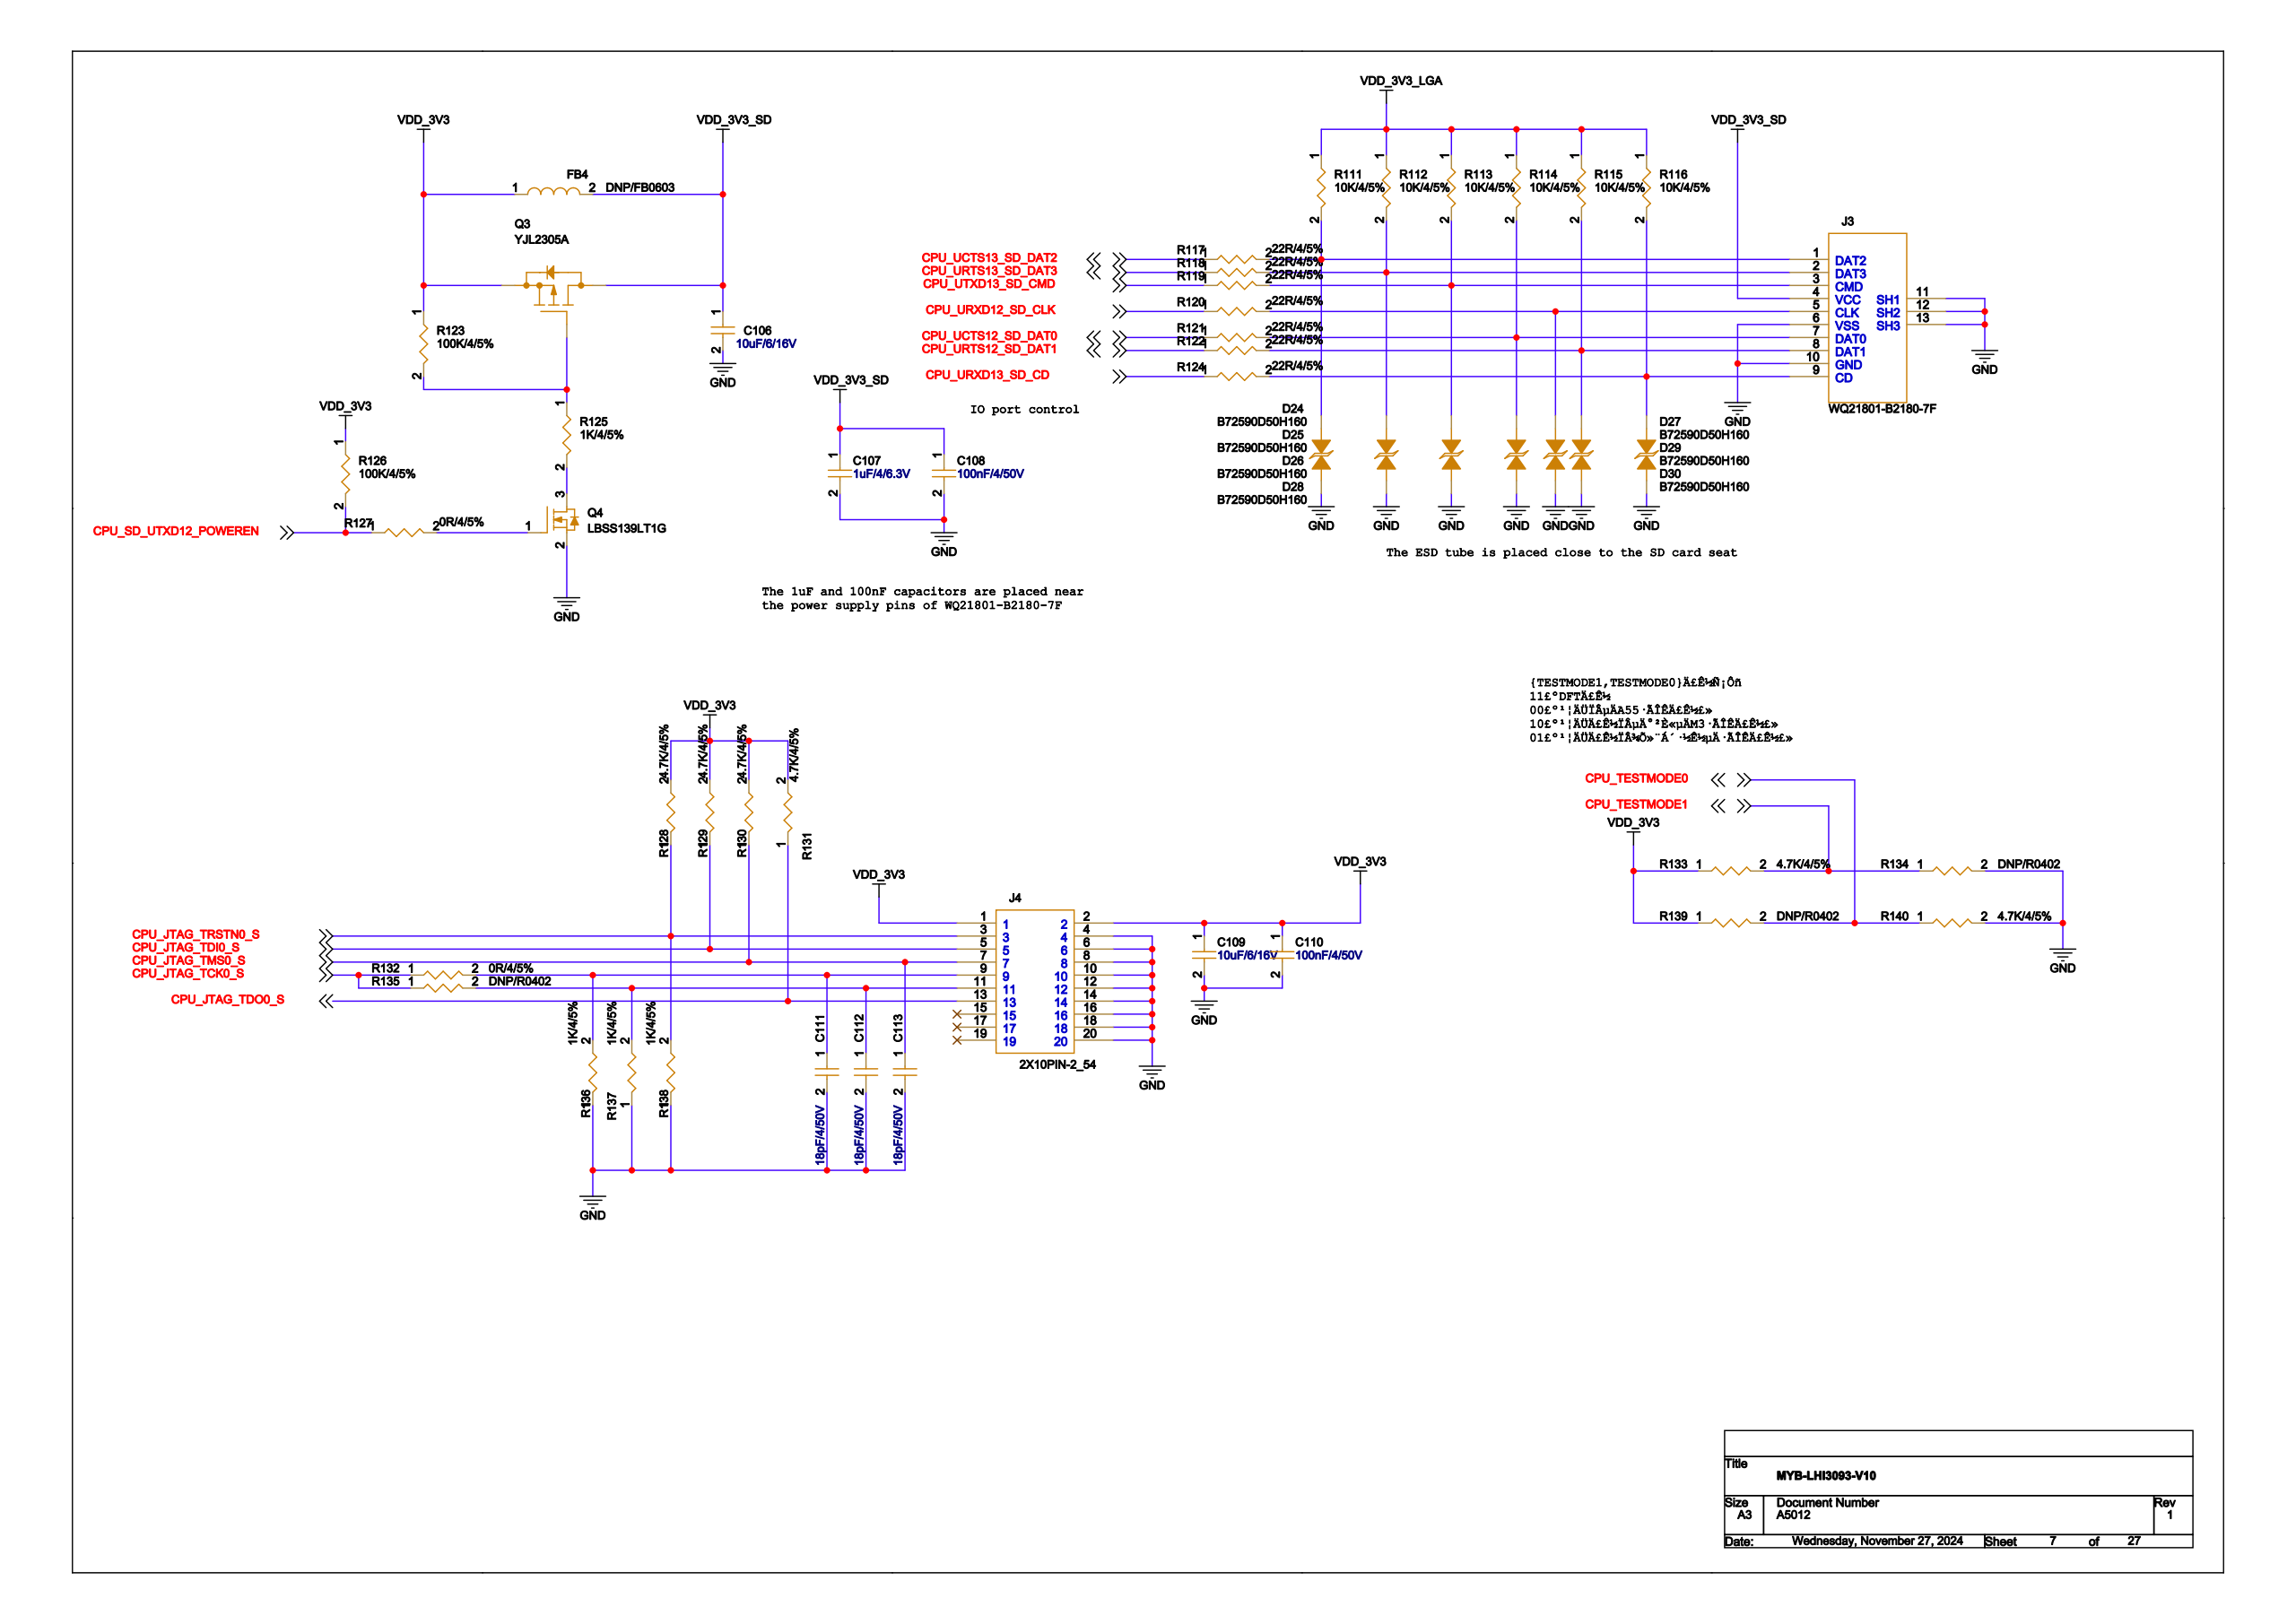Circuit board | Cadence Allegro | 1159 parts | 708 nets | one sheet of the schematic
Parts on this sheet (reference | value | footprint):
C106 | 10uF/6/16V | C0603
C107 | 1uF/4/6.3V | C0402
C108 | 100nF/4/50V | C0402
C109 | 10uF/6/16V | C0603
C110 | 100nF/4/50V | C0402
C111 | 18pF/4/50V | C0402
C112 | 18pF/4/50V | C0402
C113 | 18pF/4/50V | C0402
D24 | B72590D50H160 | D0402
D25 | B72590D50H160 | D0402
D26 | B72590D50H160 | D0402
D27 | B72590D50H160 | D0402
D28 | B72590D50H160 | D0402
D29 | B72590D50H160 | D0402
D30 | B72590D50H160 | D0402
FB4 | DNP/FB0603 | FB0603
J3 | WQ21801-B2180-7F | WQ21801-B2180-7F
J4 | 2X10PIN-2_54 | TSM-110-01-F-DV-A
Q3 | YJL2305A | SOT-23
Q4 | LBSS139LT1G | SOT-23
R111 | 10K/4/5% | R0402
R112 | 10K/4/5% | R0402
R113 | 10K/4/5% | R0402
R114 | 10K/4/5% | R0402
R115 | 10K/4/5% | R0402
R116 | 10K/4/5% | R0402
R123 | 100K/4/5% | R0402
R125 | 1K/4/5% | R0402
R126 | 100K/4/5% | R0402
R128 | 4.7K/4/5% | R0402
R129 | 4.7K/4/5% | R0402
R130 | 4.7K/4/5% | R0402
R131 | 4.7K/4/5% | R0402
R132 | 0R/4/5% | R0402
R133 | 4.7K/4/5% | R0402
R134 | DNP/R0402 | R0402
R135 | DNP/R0402 | R0402
R136 | 1K/4/5% | R0402
R137 | 1K/4/5% | R0402
R138 | 1K/4/5% | R0402
R139 | DNP/R0402 | R0402
R140 | 4.7K/4/5% | R0402
Nets of these parts (net: part-pin ...):
GND: C106-2 C107-2 C108-2 C109-2 C110-2 C111-2 C112-2 C113-2 D24-1 D25-1 D26-1 D27-1 D28-1 D29-1 D30-1 J3-6 J3-10 J3-11 J3-12 J3-13 J4-4 J4-6 J4-8 J4-10 J4-12 J4-14 J4-16 J4-18 J4-20 Q4-2 R134-2 R136-1 R137-1 R138-1 R140-2
VDD_3V3_SD: C106-1 C107-1 C108-1 FB4-2 J3-4 Q3-3
VDD_3V3: C109-1 C110-1 FB4-1 J4-1 J4-2 Q3-2 R123-1 R126-1 R128-2 R129-2 R130-2 R131-2 R133-1 R139-1
N14957727: C111-1 J4-9 R132-2 R136-2
N14957731: C112-1 J4-11 R135-2 R137-2
CPU_JTAG_TMS0_S: C113-1 J4-7 R130-1
N14955090: D24-2 J3-1 R111-2
N14955094: D25-2 J3-2 R112-2
N14955098: D26-2 J3-3 R113-2
N14955102: D27-2 J3-5
N14955106: D28-2 J3-7 R114-2
N14955110: D29-2 J3-8 R115-2
N14955114: D30-2 J3-9 R116-2
VDD_3V3_LGA: R111-1 R112-1 R113-1 R114-1 R115-1 R116-1
CPU_JTAG_TDO0_S: J4-13 R131-1
CPU_JTAG_TRSTN0_S: J4-3 R128-1 R138-2
CPU_JTAG_TDI0_S: J4-5 R129-1
N14954094: Q4-3 R125-2
N14954148: Q4-1
N14953848: Q3-1 R123-2 R125-1
CPU_SD_UTXD12_POWEREN: R126-2
CPU_JTAG_TCK0_S: R132-1 R135-1
CPU_TESTMODE1: R133-2 R134-1
CPU_TESTMODE0: R139-2 R140-1